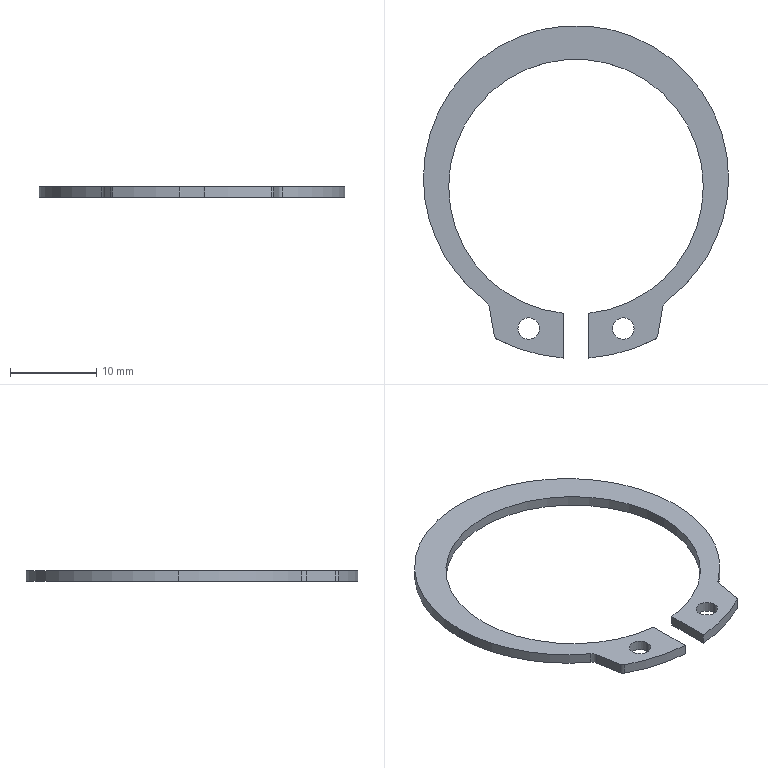Part | SolidWorks | features BaseBody 1 | 1 solid | 22 faces | box 35.48 x 38.644 x 1.2 mm | volume 408.802 mm3 | cylinder 16 | plane 6 | commonest cylinder face diameters 2.5 x4 29.6 x3 35.48 x3 1 x2 2 x2 39.96 x2
STEP:
#1=CARTESIAN_POINT('',(-4.25,-17.488,0.));
#2=VERTEX_POINT('',#1);
#3=CARTESIAN_POINT('',(-6.75,-17.488,0.));
#4=VERTEX_POINT('',#3);
#5=CARTESIAN_POINT('',(-5.5,-17.488,0.));
#6=DIRECTION('',(0.,0.,-1.));
#7=DIRECTION('',(1.,0.,0.));
#8=AXIS2_PLACEMENT_3D('',#5,#6,#7);
#9=CIRCLE('',#8,1.25);
#10=EDGE_CURVE('',#2,#4,#9,.T.);
#11=ORIENTED_EDGE('',*,*,#10,.T.);
#12=CARTESIAN_POINT('',(-6.75,-17.488,1.2));
#13=VERTEX_POINT('',#12);
#14=CARTESIAN_POINT('',(-6.75,-17.488,0.));
#15=DIRECTION('',(0.,0.,1.));
#16=VECTOR('',#15,1000.);
#17=LINE('',#14,#16);
#18=EDGE_CURVE('',#4,#13,#17,.T.);
#19=ORIENTED_EDGE('',*,*,#18,.T.);
#20=CARTESIAN_POINT('',(-4.25,-17.488,1.2));
#21=VERTEX_POINT('',#20);
#22=CARTESIAN_POINT('',(-5.5,-17.488,1.2));
#23=DIRECTION('',(0.,0.,-1.));
#24=DIRECTION('',(1.,0.,0.));
#25=AXIS2_PLACEMENT_3D('',#22,#23,#24);
#26=CIRCLE('',#25,1.25);
#27=EDGE_CURVE('',#21,#13,#26,.T.);
#28=ORIENTED_EDGE('',*,*,#27,.F.);
#29=CARTESIAN_POINT('',(-4.25,-17.488,0.));
#30=DIRECTION('',(0.,0.,1.));
#31=VECTOR('',#30,1000.);
#32=LINE('',#29,#31);
#33=EDGE_CURVE('',#2,#21,#32,.T.);
#34=ORIENTED_EDGE('',*,*,#33,.F.);
#35=EDGE_LOOP('',(#11,#19,#28,#34));
#36=FACE_OUTER_BOUND('',#35,.T.);
#37=CARTESIAN_POINT('',(-5.5,-17.488,0.));
#38=DIRECTION('',(0.,0.,1.));
#39=DIRECTION('',(1.,0.,0.));
#40=AXIS2_PLACEMENT_3D('',#37,#38,#39);
#41=CYLINDRICAL_SURFACE('',#40,1.25);
#42=ADVANCED_FACE('',(#36),#41,.F.);
#43=CARTESIAN_POINT('',(6.75,-17.488,0.));
#44=VERTEX_POINT('',#43);
#45=CARTESIAN_POINT('',(4.25,-17.488,0.));
#46=VERTEX_POINT('',#45);
#47=CARTESIAN_POINT('',(5.5,-17.488,0.));
#48=DIRECTION('',(0.,0.,-1.));
#49=DIRECTION('',(1.,0.,0.));
#50=AXIS2_PLACEMENT_3D('',#47,#48,#49);
#51=CIRCLE('',#50,1.25);
#52=EDGE_CURVE('',#44,#46,#51,.T.);
#53=ORIENTED_EDGE('',*,*,#52,.T.);
#54=CARTESIAN_POINT('',(4.25,-17.488,1.2));
#55=VERTEX_POINT('',#54);
#56=CARTESIAN_POINT('',(4.25,-17.488,0.));
#57=DIRECTION('',(0.,0.,1.));
#58=VECTOR('',#57,1000.);
#59=LINE('',#56,#58);
#60=EDGE_CURVE('',#46,#55,#59,.T.);
#61=ORIENTED_EDGE('',*,*,#60,.T.);
#62=CARTESIAN_POINT('',(6.75,-17.488,1.2));
#63=VERTEX_POINT('',#62);
#64=CARTESIAN_POINT('',(5.5,-17.488,1.2));
#65=DIRECTION('',(0.,0.,-1.));
#66=DIRECTION('',(1.,0.,0.));
#67=AXIS2_PLACEMENT_3D('',#64,#65,#66);
#68=CIRCLE('',#67,1.25);
#69=EDGE_CURVE('',#63,#55,#68,.T.);
#70=ORIENTED_EDGE('',*,*,#69,.F.);
#71=CARTESIAN_POINT('',(6.75,-17.488,0.));
#72=DIRECTION('',(0.,0.,1.));
#73=VECTOR('',#72,1000.);
#74=LINE('',#71,#73);
#75=EDGE_CURVE('',#44,#63,#74,.T.);
#76=ORIENTED_EDGE('',*,*,#75,.F.);
#77=EDGE_LOOP('',(#53,#61,#70,#76));
#78=FACE_OUTER_BOUND('',#77,.T.);
#79=CARTESIAN_POINT('',(5.5,-17.488,0.));
#80=DIRECTION('',(0.,0.,1.));
#81=DIRECTION('',(1.,0.,0.));
#82=AXIS2_PLACEMENT_3D('',#79,#80,#81);
#83=CYLINDRICAL_SURFACE('',#82,1.25);
#84=ADVANCED_FACE('',(#78),#83,.F.);
#85=CARTESIAN_POINT('',(17.74,0.,0.));
#86=VERTEX_POINT('',#85);
#87=CARTESIAN_POINT('',(-17.74,0.,0.));
#88=VERTEX_POINT('',#87);
#89=CARTESIAN_POINT('',(0.,0.,0.));
#90=DIRECTION('',(0.,0.,1.));
#91=DIRECTION('',(1.,0.,0.));
#92=AXIS2_PLACEMENT_3D('',#89,#90,#91);
#93=CIRCLE('',#92,17.74);
#94=EDGE_CURVE('',#86,#88,#93,.T.);
#95=ORIENTED_EDGE('',*,*,#94,.T.);
#96=CARTESIAN_POINT('',(-17.74,0.,1.2));
#97=VERTEX_POINT('',#96);
#98=CARTESIAN_POINT('',(-17.74,0.,0.));
#99=DIRECTION('',(0.,0.,1.));
#100=VECTOR('',#99,1000.);
#101=LINE('',#98,#100);
#102=EDGE_CURVE('',#88,#97,#101,.T.);
#103=ORIENTED_EDGE('',*,*,#102,.T.);
#104=CARTESIAN_POINT('',(17.74,0.,1.2));
#105=VERTEX_POINT('',#104);
#106=CARTESIAN_POINT('',(0.,0.,1.2));
#107=DIRECTION('',(0.,0.,-1.));
#108=DIRECTION('',(1.,0.,0.));
#109=AXIS2_PLACEMENT_3D('',#106,#107,#108);
#110=CIRCLE('',#109,17.74);
#111=EDGE_CURVE('',#97,#105,#110,.T.);
#112=ORIENTED_EDGE('',*,*,#111,.T.);
#113=CARTESIAN_POINT('',(17.74,0.,0.));
#114=DIRECTION('',(0.,0.,1.));
#115=VECTOR('',#114,1000.);
#116=LINE('',#113,#115);
#117=EDGE_CURVE('',#86,#105,#116,.T.);
#118=ORIENTED_EDGE('',*,*,#117,.F.);
#119=EDGE_LOOP('',(#95,#103,#112,#118));
#120=FACE_OUTER_BOUND('',#119,.T.);
#121=CARTESIAN_POINT('',(0.,0.,0.));
#122=DIRECTION('',(0.,0.,1.));
#123=DIRECTION('',(1.,0.,0.));
#124=AXIS2_PLACEMENT_3D('',#121,#122,#123);
#125=CYLINDRICAL_SURFACE('',#124,17.74);
#126=ADVANCED_FACE('',(#120),#125,.T.);
#127=CARTESIAN_POINT('',(10.493,-14.304,0.));
#128=VERTEX_POINT('',#127);
#129=CARTESIAN_POINT('',(0.,0.,0.));
#130=DIRECTION('',(0.,0.,1.));
#131=DIRECTION('',(1.,0.,0.));
#132=AXIS2_PLACEMENT_3D('',#129,#130,#131);
#133=CIRCLE('',#132,17.74);
#134=EDGE_CURVE('',#128,#86,#133,.T.);
#135=ORIENTED_EDGE('',*,*,#134,.T.);
#136=ORIENTED_EDGE('',*,*,#117,.T.);
#137=CARTESIAN_POINT('',(10.493,-14.304,1.2));
#138=VERTEX_POINT('',#137);
#139=CARTESIAN_POINT('',(0.,0.,1.2));
#140=DIRECTION('',(0.,0.,-1.));
#141=DIRECTION('',(1.,0.,0.));
#142=AXIS2_PLACEMENT_3D('',#139,#140,#141);
#143=CIRCLE('',#142,17.74);
#144=EDGE_CURVE('',#105,#138,#143,.T.);
#145=ORIENTED_EDGE('',*,*,#144,.T.);
#146=CARTESIAN_POINT('',(10.493,-14.304,0.));
#147=DIRECTION('',(0.,0.,-1.));
#148=VECTOR('',#147,1000.);
#149=LINE('',#146,#148);
#150=EDGE_CURVE('',#138,#128,#149,.T.);
#151=ORIENTED_EDGE('',*,*,#150,.T.);
#152=EDGE_LOOP('',(#135,#136,#145,#151));
#153=FACE_OUTER_BOUND('',#152,.T.);
#154=CARTESIAN_POINT('',(0.,0.,0.));
#155=DIRECTION('',(0.,0.,1.));
#156=DIRECTION('',(1.,0.,0.));
#157=AXIS2_PLACEMENT_3D('',#154,#155,#156);
#158=CYLINDRICAL_SURFACE('',#157,17.74);
#159=ADVANCED_FACE('',(#153),#158,.T.);
#160=CARTESIAN_POINT('',(-1.5,-15.704,0.));
#161=VERTEX_POINT('',#160);
#162=CARTESIAN_POINT('',(-14.8,-0.98,0.));
#163=VERTEX_POINT('',#162);
#164=CARTESIAN_POINT('',(0.,-0.98,0.));
#165=DIRECTION('',(0.,0.,-1.));
#166=DIRECTION('',(1.,0.,0.));
#167=AXIS2_PLACEMENT_3D('',#164,#165,#166);
#168=CIRCLE('',#167,14.8);
#169=EDGE_CURVE('',#161,#163,#168,.T.);
#170=ORIENTED_EDGE('',*,*,#169,.T.);
#171=CARTESIAN_POINT('',(-14.8,-0.98,1.2));
#172=VERTEX_POINT('',#171);
#173=CARTESIAN_POINT('',(-14.8,-0.98,0.));
#174=DIRECTION('',(0.,0.,1.));
#175=VECTOR('',#174,1000.);
#176=LINE('',#173,#175);
#177=EDGE_CURVE('',#163,#172,#176,.T.);
#178=ORIENTED_EDGE('',*,*,#177,.T.);
#179=CARTESIAN_POINT('',(-1.5,-15.704,1.2));
#180=VERTEX_POINT('',#179);
#181=CARTESIAN_POINT('',(0.,-0.98,1.2));
#182=DIRECTION('',(0.,0.,-1.));
#183=DIRECTION('',(1.,0.,0.));
#184=AXIS2_PLACEMENT_3D('',#181,#182,#183);
#185=CIRCLE('',#184,14.8);
#186=EDGE_CURVE('',#180,#172,#185,.T.);
#187=ORIENTED_EDGE('',*,*,#186,.F.);
#188=CARTESIAN_POINT('',(-1.5,-15.704,0.));
#189=DIRECTION('',(0.,0.,1.));
#190=VECTOR('',#189,1000.);
#191=LINE('',#188,#190);
#192=EDGE_CURVE('',#161,#180,#191,.T.);
#193=ORIENTED_EDGE('',*,*,#192,.F.);
#194=EDGE_LOOP('',(#170,#178,#187,#193));
#195=FACE_OUTER_BOUND('',#194,.T.);
#196=CARTESIAN_POINT('',(0.,-0.98,0.));
#197=DIRECTION('',(0.,0.,1.));
#198=DIRECTION('',(1.,0.,0.));
#199=AXIS2_PLACEMENT_3D('',#196,#197,#198);
#200=CYLINDRICAL_SURFACE('',#199,14.8);
#201=ADVANCED_FACE('',(#195),#200,.F.);
#202=ORIENTED_EDGE('',*,*,#177,.F.);
#203=CARTESIAN_POINT('',(14.8,-0.98,0.));
#204=VERTEX_POINT('',#203);
#205=CARTESIAN_POINT('',(0.,-0.98,0.));
#206=DIRECTION('',(0.,0.,-1.));
#207=DIRECTION('',(1.,0.,0.));
#208=AXIS2_PLACEMENT_3D('',#205,#206,#207);
#209=CIRCLE('',#208,14.8);
#210=EDGE_CURVE('',#163,#204,#209,.T.);
#211=ORIENTED_EDGE('',*,*,#210,.T.);
#212=CARTESIAN_POINT('',(14.8,-0.98,1.2));
#213=VERTEX_POINT('',#212);
#214=CARTESIAN_POINT('',(14.8,-0.98,0.));
#215=DIRECTION('',(0.,0.,1.));
#216=VECTOR('',#215,1000.);
#217=LINE('',#214,#216);
#218=EDGE_CURVE('',#204,#213,#217,.T.);
#219=ORIENTED_EDGE('',*,*,#218,.T.);
#220=CARTESIAN_POINT('',(0.,-0.98,1.2));
#221=DIRECTION('',(0.,0.,-1.));
#222=DIRECTION('',(1.,0.,0.));
#223=AXIS2_PLACEMENT_3D('',#220,#221,#222);
#224=CIRCLE('',#223,14.8);
#225=EDGE_CURVE('',#172,#213,#224,.T.);
#226=ORIENTED_EDGE('',*,*,#225,.F.);
#227=EDGE_LOOP('',(#202,#211,#219,#226));
#228=FACE_OUTER_BOUND('',#227,.T.);
#229=CARTESIAN_POINT('',(0.,-0.98,0.));
#230=DIRECTION('',(0.,0.,1.));
#231=DIRECTION('',(1.,0.,0.));
#232=AXIS2_PLACEMENT_3D('',#229,#230,#231);
#233=CYLINDRICAL_SURFACE('',#232,14.8);
#234=ADVANCED_FACE('',(#228),#233,.F.);
#235=ORIENTED_EDGE('',*,*,#10,.F.);
#236=CARTESIAN_POINT('',(-5.5,-17.488,0.));
#237=DIRECTION('',(0.,0.,-1.));
#238=DIRECTION('',(1.,0.,0.));
#239=AXIS2_PLACEMENT_3D('',#236,#237,#238);
#240=CIRCLE('',#239,1.25);
#241=EDGE_CURVE('',#4,#2,#240,.T.);
#242=ORIENTED_EDGE('',*,*,#241,.F.);
#243=EDGE_LOOP('',(#235,#242));
#244=FACE_BOUND('',#243,.T.);
#245=ORIENTED_EDGE('',*,*,#52,.F.);
#246=CARTESIAN_POINT('',(5.5,-17.488,0.));
#247=DIRECTION('',(0.,0.,-1.));
#248=DIRECTION('',(1.,0.,0.));
#249=AXIS2_PLACEMENT_3D('',#246,#247,#248);
#250=CIRCLE('',#249,1.25);
#251=EDGE_CURVE('',#46,#44,#250,.T.);
#252=ORIENTED_EDGE('',*,*,#251,.F.);
#253=EDGE_LOOP('',(#245,#252));
#254=FACE_BOUND('',#253,.T.);
#255=CARTESIAN_POINT('',(-9.5,-18.339,0.));
#256=VERTEX_POINT('',#255);
#257=CARTESIAN_POINT('',(-9.239,-18.696,0.));
#258=VERTEX_POINT('',#257);
#259=CARTESIAN_POINT('',(-9.008,-18.253,0.));
#260=DIRECTION('',(0.,0.,1.));
#261=DIRECTION('',(1.,0.,0.));
#262=AXIS2_PLACEMENT_3D('',#259,#260,#261);
#263=CIRCLE('',#262,0.5);
#264=EDGE_CURVE('',#256,#258,#263,.T.);
#265=ORIENTED_EDGE('',*,*,#264,.F.);
#266=CARTESIAN_POINT('',(-10.1,-14.936,0.));
#267=VERTEX_POINT('',#266);
#268=CARTESIAN_POINT('',(-10.1,-14.936,0.));
#269=DIRECTION('',(0.1736,-0.9848,0.));
#270=VECTOR('',#269,1000.);
#271=LINE('',#268,#270);
#272=EDGE_CURVE('',#267,#256,#271,.T.);
#273=ORIENTED_EDGE('',*,*,#272,.F.);
#274=CARTESIAN_POINT('',(-10.493,-14.304,0.));
#275=VERTEX_POINT('',#274);
#276=CARTESIAN_POINT('',(-11.085,-15.11,0.));
#277=DIRECTION('',(0.,0.,-1.));
#278=DIRECTION('',(1.,0.,0.));
#279=AXIS2_PLACEMENT_3D('',#276,#277,#278);
#280=CIRCLE('',#279,1.);
#281=EDGE_CURVE('',#275,#267,#280,.T.);
#282=ORIENTED_EDGE('',*,*,#281,.F.);
#283=CARTESIAN_POINT('',(0.,0.,0.));
#284=DIRECTION('',(0.,0.,1.));
#285=DIRECTION('',(1.,0.,0.));
#286=AXIS2_PLACEMENT_3D('',#283,#284,#285);
#287=CIRCLE('',#286,17.74);
#288=EDGE_CURVE('',#88,#275,#287,.T.);
#289=ORIENTED_EDGE('',*,*,#288,.F.);
#290=ORIENTED_EDGE('',*,*,#94,.F.);
#291=ORIENTED_EDGE('',*,*,#134,.F.);
#292=CARTESIAN_POINT('',(10.1,-14.936,0.));
#293=VERTEX_POINT('',#292);
#294=CARTESIAN_POINT('',(11.085,-15.11,0.));
#295=DIRECTION('',(0.,0.,-1.));
#296=DIRECTION('',(1.,0.,0.));
#297=AXIS2_PLACEMENT_3D('',#294,#295,#296);
#298=CIRCLE('',#297,1.);
#299=EDGE_CURVE('',#293,#128,#298,.T.);
#300=ORIENTED_EDGE('',*,*,#299,.F.);
#301=CARTESIAN_POINT('',(9.5,-18.339,0.));
#302=VERTEX_POINT('',#301);
#303=CARTESIAN_POINT('',(9.5,-18.339,0.));
#304=DIRECTION('',(0.1736,0.9848,0.));
#305=VECTOR('',#304,1000.);
#306=LINE('',#303,#305);
#307=EDGE_CURVE('',#302,#293,#306,.T.);
#308=ORIENTED_EDGE('',*,*,#307,.F.);
#309=CARTESIAN_POINT('',(9.239,-18.696,0.));
#310=VERTEX_POINT('',#309);
#311=CARTESIAN_POINT('',(9.008,-18.253,0.));
#312=DIRECTION('',(0.,0.,1.));
#313=DIRECTION('',(1.,0.,0.));
#314=AXIS2_PLACEMENT_3D('',#311,#312,#313);
#315=CIRCLE('',#314,0.5);
#316=EDGE_CURVE('',#310,#302,#315,.T.);
#317=ORIENTED_EDGE('',*,*,#316,.F.);
#318=CARTESIAN_POINT('',(1.5,-20.904,0.));
#319=VERTEX_POINT('',#318);
#320=CARTESIAN_POINT('',(0.,-0.98,0.));
#321=DIRECTION('',(0.,0.,1.));
#322=DIRECTION('',(1.,0.,0.));
#323=AXIS2_PLACEMENT_3D('',#320,#321,#322);
#324=CIRCLE('',#323,19.98);
#325=EDGE_CURVE('',#319,#310,#324,.T.);
#326=ORIENTED_EDGE('',*,*,#325,.F.);
#327=CARTESIAN_POINT('',(1.5,-15.704,0.));
#328=VERTEX_POINT('',#327);
#329=CARTESIAN_POINT('',(1.5,-2.899,0.));
#330=DIRECTION('',(0.,-1.,0.));
#331=VECTOR('',#330,1000.);
#332=LINE('',#329,#331);
#333=EDGE_CURVE('',#328,#319,#332,.T.);
#334=ORIENTED_EDGE('',*,*,#333,.F.);
#335=CARTESIAN_POINT('',(0.,-0.98,0.));
#336=DIRECTION('',(0.,0.,-1.));
#337=DIRECTION('',(1.,0.,0.));
#338=AXIS2_PLACEMENT_3D('',#335,#336,#337);
#339=CIRCLE('',#338,14.8);
#340=EDGE_CURVE('',#204,#328,#339,.T.);
#341=ORIENTED_EDGE('',*,*,#340,.F.);
#342=ORIENTED_EDGE('',*,*,#210,.F.);
#343=ORIENTED_EDGE('',*,*,#169,.F.);
#344=CARTESIAN_POINT('',(-1.5,-20.904,0.));
#345=VERTEX_POINT('',#344);
#346=CARTESIAN_POINT('',(-1.5,-2.899,0.));
#347=DIRECTION('',(0.,1.,0.));
#348=VECTOR('',#347,1000.);
#349=LINE('',#346,#348);
#350=EDGE_CURVE('',#345,#161,#349,.T.);
#351=ORIENTED_EDGE('',*,*,#350,.F.);
#352=CARTESIAN_POINT('',(0.,-0.98,0.));
#353=DIRECTION('',(0.,0.,1.));
#354=DIRECTION('',(1.,0.,0.));
#355=AXIS2_PLACEMENT_3D('',#352,#353,#354);
#356=CIRCLE('',#355,19.98);
#357=EDGE_CURVE('',#258,#345,#356,.T.);
#358=ORIENTED_EDGE('',*,*,#357,.F.);
#359=EDGE_LOOP('',(#265,#273,#282,#289,#290,#291,#300,#308,#317,#326,#334,#341,#342,#343,#351,#358));
#360=FACE_OUTER_BOUND('',#359,.T.);
#361=CARTESIAN_POINT('',(0.,-2.899,0.));
#362=DIRECTION('',(0.,0.,1.));
#363=DIRECTION('',(1.,0.,0.));
#364=AXIS2_PLACEMENT_3D('',#361,#362,#363);
#365=PLANE('',#364);
#366=ADVANCED_FACE('',(#244,#254,#360),#365,.F.);
#367=ORIENTED_EDGE('',*,*,#18,.F.);
#368=ORIENTED_EDGE('',*,*,#241,.T.);
#369=ORIENTED_EDGE('',*,*,#33,.T.);
#370=CARTESIAN_POINT('',(-5.5,-17.488,1.2));
#371=DIRECTION('',(0.,0.,-1.));
#372=DIRECTION('',(1.,0.,0.));
#373=AXIS2_PLACEMENT_3D('',#370,#371,#372);
#374=CIRCLE('',#373,1.25);
#375=EDGE_CURVE('',#13,#21,#374,.T.);
#376=ORIENTED_EDGE('',*,*,#375,.F.);
#377=EDGE_LOOP('',(#367,#368,#369,#376));
#378=FACE_OUTER_BOUND('',#377,.T.);
#379=CARTESIAN_POINT('',(-5.5,-17.488,0.));
#380=DIRECTION('',(0.,0.,1.));
#381=DIRECTION('',(1.,0.,0.));
#382=AXIS2_PLACEMENT_3D('',#379,#380,#381);
#383=CYLINDRICAL_SURFACE('',#382,1.25);
#384=ADVANCED_FACE('',(#378),#383,.F.);
#385=ORIENTED_EDGE('',*,*,#60,.F.);
#386=ORIENTED_EDGE('',*,*,#251,.T.);
#387=ORIENTED_EDGE('',*,*,#75,.T.);
#388=CARTESIAN_POINT('',(5.5,-17.488,1.2));
#389=DIRECTION('',(0.,0.,-1.));
#390=DIRECTION('',(1.,0.,0.));
#391=AXIS2_PLACEMENT_3D('',#388,#389,#390);
#392=CIRCLE('',#391,1.25);
#393=EDGE_CURVE('',#55,#63,#392,.T.);
#394=ORIENTED_EDGE('',*,*,#393,.F.);
#395=EDGE_LOOP('',(#385,#386,#387,#394));
#396=FACE_OUTER_BOUND('',#395,.T.);
#397=CARTESIAN_POINT('',(5.5,-17.488,0.));
#398=DIRECTION('',(0.,0.,1.));
#399=DIRECTION('',(1.,0.,0.));
#400=AXIS2_PLACEMENT_3D('',#397,#398,#399);
#401=CYLINDRICAL_SURFACE('',#400,1.25);
#402=ADVANCED_FACE('',(#396),#401,.F.);
#403=ORIENTED_EDGE('',*,*,#357,.T.);
#404=CARTESIAN_POINT('',(-1.5,-20.904,1.2));
#405=VERTEX_POINT('',#404);
#406=CARTESIAN_POINT('',(-1.5,-20.904,0.));
#407=DIRECTION('',(0.,0.,1.));
#408=VECTOR('',#407,1000.);
#409=LINE('',#406,#408);
#410=EDGE_CURVE('',#345,#405,#409,.T.);
#411=ORIENTED_EDGE('',*,*,#410,.T.);
#412=CARTESIAN_POINT('',(-9.239,-18.696,1.2));
#413=VERTEX_POINT('',#412);
#414=CARTESIAN_POINT('',(0.,-0.98,1.2));
#415=DIRECTION('',(0.,0.,-1.));
#416=DIRECTION('',(1.,0.,0.));
#417=AXIS2_PLACEMENT_3D('',#414,#415,#416);
#418=CIRCLE('',#417,19.98);
#419=EDGE_CURVE('',#405,#413,#418,.T.);
#420=ORIENTED_EDGE('',*,*,#419,.T.);
#421=CARTESIAN_POINT('',(-9.239,-18.696,0.));
#422=DIRECTION('',(0.,0.,-1.));
#423=VECTOR('',#422,1000.);
#424=LINE('',#421,#423);
#425=EDGE_CURVE('',#413,#258,#424,.T.);
#426=ORIENTED_EDGE('',*,*,#425,.T.);
#427=EDGE_LOOP('',(#403,#411,#420,#426));
#428=FACE_OUTER_BOUND('',#427,.T.);
#429=CARTESIAN_POINT('',(0.,-0.98,0.));
#430=DIRECTION('',(0.,0.,1.));
#431=DIRECTION('',(1.,0.,0.));
#432=AXIS2_PLACEMENT_3D('',#429,#430,#431);
#433=CYLINDRICAL_SURFACE('',#432,19.98);
#434=ADVANCED_FACE('',(#428),#433,.T.);
#435=ORIENTED_EDGE('',*,*,#264,.T.);
#436=ORIENTED_EDGE('',*,*,#425,.F.);
#437=CARTESIAN_POINT('',(-9.5,-18.339,1.2));
#438=VERTEX_POINT('',#437);
#439=CARTESIAN_POINT('',(-9.008,-18.253,1.2));
#440=DIRECTION('',(0.,0.,-1.));
#441=DIRECTION('',(1.,0.,0.));
#442=AXIS2_PLACEMENT_3D('',#439,#440,#441);
#443=CIRCLE('',#442,0.5);
#444=EDGE_CURVE('',#413,#438,#443,.T.);
#445=ORIENTED_EDGE('',*,*,#444,.T.);
#446=CARTESIAN_POINT('',(-9.5,-18.339,0.));
#447=DIRECTION('',(0.,0.,-1.));
#448=VECTOR('',#447,1000.);
#449=LINE('',#446,#448);
#450=EDGE_CURVE('',#438,#256,#449,.T.);
#451=ORIENTED_EDGE('',*,*,#450,.T.);
#452=EDGE_LOOP('',(#435,#436,#445,#451));
#453=FACE_OUTER_BOUND('',#452,.T.);
#454=CARTESIAN_POINT('',(-9.008,-18.253,0.));
#455=DIRECTION('',(0.,0.,1.));
#456=DIRECTION('',(1.,0.,0.));
#457=AXIS2_PLACEMENT_3D('',#454,#455,#456);
#458=CYLINDRICAL_SURFACE('',#457,0.5);
#459=ADVANCED_FACE('',(#453),#458,.T.);
#460=ORIENTED_EDGE('',*,*,#272,.T.);
#461=ORIENTED_EDGE('',*,*,#450,.F.);
#462=CARTESIAN_POINT('',(-10.1,-14.936,1.2));
#463=VERTEX_POINT('',#462);
#464=CARTESIAN_POINT('',(-9.5,-18.339,1.2));
#465=DIRECTION('',(-0.1736,0.9848,0.));
#466=VECTOR('',#465,1000.);
#467=LINE('',#464,#466);
#468=EDGE_CURVE('',#438,#463,#467,.T.);
#469=ORIENTED_EDGE('',*,*,#468,.T.);
#470=CARTESIAN_POINT('',(-10.1,-14.936,0.));
#471=DIRECTION('',(0.,0.,-1.));
#472=VECTOR('',#471,1000.);
#473=LINE('',#470,#472);
#474=EDGE_CURVE('',#463,#267,#473,.T.);
#475=ORIENTED_EDGE('',*,*,#474,.T.);
#476=EDGE_LOOP('',(#460,#461,#469,#475));
#477=FACE_OUTER_BOUND('',#476,.T.);
#478=CARTESIAN_POINT('',(-9.5,-18.339,0.));
#479=DIRECTION('',(-0.9848,-0.1736,0.));
#480=DIRECTION('',(0.1736,-0.9848,0.));
#481=AXIS2_PLACEMENT_3D('',#478,#479,#480);
#482=PLANE('',#481);
#483=ADVANCED_FACE('',(#477),#482,.T.);
#484=CARTESIAN_POINT('',(-10.493,-14.304,1.2));
#485=VERTEX_POINT('',#484);
#486=CARTESIAN_POINT('',(-10.493,-14.304,0.));
#487=DIRECTION('',(0.,0.,1.));
#488=VECTOR('',#487,1000.);
#489=LINE('',#486,#488);
#490=EDGE_CURVE('',#275,#485,#489,.T.);
#491=ORIENTED_EDGE('',*,*,#490,.F.);
#492=ORIENTED_EDGE('',*,*,#281,.T.);
#493=ORIENTED_EDGE('',*,*,#474,.F.);
#494=CARTESIAN_POINT('',(-11.085,-15.11,1.2));
#495=DIRECTION('',(0.,0.,-1.));
#496=DIRECTION('',(1.,0.,0.));
#497=AXIS2_PLACEMENT_3D('',#494,#495,#496);
#498=CIRCLE('',#497,1.);
#499=EDGE_CURVE('',#485,#463,#498,.T.);
#500=ORIENTED_EDGE('',*,*,#499,.F.);
#501=EDGE_LOOP('',(#491,#492,#493,#500));
#502=FACE_OUTER_BOUND('',#501,.T.);
#503=CARTESIAN_POINT('',(-11.085,-15.11,0.));
#504=DIRECTION('',(0.,0.,1.));
#505=DIRECTION('',(1.,0.,0.));
#506=AXIS2_PLACEMENT_3D('',#503,#504,#505);
#507=CYLINDRICAL_SURFACE('',#506,1.);
#508=ADVANCED_FACE('',(#502),#507,.F.);
#509=ORIENTED_EDGE('',*,*,#102,.F.);
#510=ORIENTED_EDGE('',*,*,#288,.T.);
#511=ORIENTED_EDGE('',*,*,#490,.T.);
#512=CARTESIAN_POINT('',(0.,0.,1.2));
#513=DIRECTION('',(0.,0.,-1.));
#514=DIRECTION('',(1.,0.,0.));
#515=AXIS2_PLACEMENT_3D('',#512,#513,#514);
#516=CIRCLE('',#515,17.74);
#517=EDGE_CURVE('',#485,#97,#516,.T.);
#518=ORIENTED_EDGE('',*,*,#517,.T.);
#519=EDGE_LOOP('',(#509,#510,#511,#518));
#520=FACE_OUTER_BOUND('',#519,.T.);
#521=CARTESIAN_POINT('',(0.,0.,0.));
#522=DIRECTION('',(0.,0.,1.));
#523=DIRECTION('',(1.,0.,0.));
#524=AXIS2_PLACEMENT_3D('',#521,#522,#523);
#525=CYLINDRICAL_SURFACE('',#524,17.74);
#526=ADVANCED_FACE('',(#520),#525,.T.);
#527=CARTESIAN_POINT('',(10.1,-14.936,1.2));
#528=VERTEX_POINT('',#527);
#529=CARTESIAN_POINT('',(10.1,-14.936,0.));
#530=DIRECTION('',(0.,0.,1.));
#531=VECTOR('',#530,1000.);
#532=LINE('',#529,#531);
#533=EDGE_CURVE('',#293,#528,#532,.T.);
#534=ORIENTED_EDGE('',*,*,#533,.F.);
#535=ORIENTED_EDGE('',*,*,#299,.T.);
#536=ORIENTED_EDGE('',*,*,#150,.F.);
#537=CARTESIAN_POINT('',(11.085,-15.11,1.2));
#538=DIRECTION('',(0.,0.,-1.));
#539=DIRECTION('',(1.,0.,0.));
#540=AXIS2_PLACEMENT_3D('',#537,#538,#539);
#541=CIRCLE('',#540,1.);
#542=EDGE_CURVE('',#528,#138,#541,.T.);
#543=ORIENTED_EDGE('',*,*,#542,.F.);
#544=EDGE_LOOP('',(#534,#535,#536,#543));
#545=FACE_OUTER_BOUND('',#544,.T.);
#546=CARTESIAN_POINT('',(11.085,-15.11,0.));
#547=DIRECTION('',(0.,0.,1.));
#548=DIRECTION('',(1.,0.,0.));
#549=AXIS2_PLACEMENT_3D('',#546,#547,#548);
#550=CYLINDRICAL_SURFACE('',#549,1.);
#551=ADVANCED_FACE('',(#545),#550,.F.);
#552=ORIENTED_EDGE('',*,*,#307,.T.);
#553=ORIENTED_EDGE('',*,*,#533,.T.);
#554=CARTESIAN_POINT('',(9.5,-18.339,1.2));
#555=VERTEX_POINT('',#554);
#556=CARTESIAN_POINT('',(10.1,-14.936,1.2));
#557=DIRECTION('',(-0.1736,-0.9848,0.));
#558=VECTOR('',#557,1000.);
#559=LINE('',#556,#558);
#560=EDGE_CURVE('',#528,#555,#559,.T.);
#561=ORIENTED_EDGE('',*,*,#560,.T.);
#562=CARTESIAN_POINT('',(9.5,-18.339,0.));
#563=DIRECTION('',(0.,0.,-1.));
#564=VECTOR('',#563,1000.);
#565=LINE('',#562,#564);
#566=EDGE_CURVE('',#555,#302,#565,.T.);
#567=ORIENTED_EDGE('',*,*,#566,.T.);
#568=EDGE_LOOP('',(#552,#553,#561,#567));
#569=FACE_OUTER_BOUND('',#568,.T.);
#570=CARTESIAN_POINT('',(10.1,-14.936,0.));
#571=DIRECTION('',(0.9848,-0.1736,0.));
#572=DIRECTION('',(0.1736,0.9848,0.));
#573=AXIS2_PLACEMENT_3D('',#570,#571,#572);
#574=PLANE('',#573);
#575=ADVANCED_FACE('',(#569),#574,.T.);
#576=ORIENTED_EDGE('',*,*,#316,.T.);
#577=ORIENTED_EDGE('',*,*,#566,.F.);
#578=CARTESIAN_POINT('',(9.239,-18.696,1.2));
#579=VERTEX_POINT('',#578);
#580=CARTESIAN_POINT('',(9.008,-18.253,1.2));
#581=DIRECTION('',(0.,0.,-1.));
#582=DIRECTION('',(1.,0.,0.));
#583=AXIS2_PLACEMENT_3D('',#580,#581,#582);
#584=CIRCLE('',#583,0.5);
#585=EDGE_CURVE('',#555,#579,#584,.T.);
#586=ORIENTED_EDGE('',*,*,#585,.T.);
#587=CARTESIAN_POINT('',(9.239,-18.696,0.));
#588=DIRECTION('',(0.,0.,-1.));
#589=VECTOR('',#588,1000.);
#590=LINE('',#587,#589);
#591=EDGE_CURVE('',#579,#310,#590,.T.);
#592=ORIENTED_EDGE('',*,*,#591,.T.);
#593=EDGE_LOOP('',(#576,#577,#586,#592));
#594=FACE_OUTER_BOUND('',#593,.T.);
#595=CARTESIAN_POINT('',(9.008,-18.253,0.));
#596=DIRECTION('',(0.,0.,1.));
#597=DIRECTION('',(1.,0.,0.));
#598=AXIS2_PLACEMENT_3D('',#595,#596,#597);
#599=CYLINDRICAL_SURFACE('',#598,0.5);
#600=ADVANCED_FACE('',(#594),#599,.T.);
#601=ORIENTED_EDGE('',*,*,#325,.T.);
#602=ORIENTED_EDGE('',*,*,#591,.F.);
#603=CARTESIAN_POINT('',(1.5,-20.904,1.2));
#604=VERTEX_POINT('',#603);
#605=CARTESIAN_POINT('',(0.,-0.98,1.2));
#606=DIRECTION('',(0.,0.,-1.));
#607=DIRECTION('',(1.,0.,0.));
#608=AXIS2_PLACEMENT_3D('',#605,#606,#607);
#609=CIRCLE('',#608,19.98);
#610=EDGE_CURVE('',#579,#604,#609,.T.);
#611=ORIENTED_EDGE('',*,*,#610,.T.);
#612=CARTESIAN_POINT('',(1.5,-20.904,0.));
#613=DIRECTION('',(0.,0.,-1.));
#614=VECTOR('',#613,1000.);
#615=LINE('',#612,#614);
#616=EDGE_CURVE('',#604,#319,#615,.T.);
#617=ORIENTED_EDGE('',*,*,#616,.T.);
#618=EDGE_LOOP('',(#601,#602,#611,#617));
#619=FACE_OUTER_BOUND('',#618,.T.);
#620=CARTESIAN_POINT('',(0.,-0.98,0.));
#621=DIRECTION('',(0.,0.,1.));
#622=DIRECTION('',(1.,0.,0.));
#623=AXIS2_PLACEMENT_3D('',#620,#621,#622);
#624=CYLINDRICAL_SURFACE('',#623,19.98);
#625=ADVANCED_FACE('',(#619),#624,.T.);
#626=ORIENTED_EDGE('',*,*,#333,.T.);
#627=ORIENTED_EDGE('',*,*,#616,.F.);
#628=CARTESIAN_POINT('',(1.5,-15.704,1.2));
#629=VERTEX_POINT('',#628);
#630=CARTESIAN_POINT('',(1.5,-20.904,1.2));
#631=DIRECTION('',(0.,1.,0.));
#632=VECTOR('',#631,1000.);
#633=LINE('',#630,#632);
#634=EDGE_CURVE('',#604,#629,#633,.T.);
#635=ORIENTED_EDGE('',*,*,#634,.T.);
#636=CARTESIAN_POINT('',(1.5,-15.704,0.));
#637=DIRECTION('',(0.,0.,-1.));
#638=VECTOR('',#637,1000.);
#639=LINE('',#636,#638);
#640=EDGE_CURVE('',#629,#328,#639,.T.);
#641=ORIENTED_EDGE('',*,*,#640,.T.);
#642=EDGE_LOOP('',(#626,#627,#635,#641));
#643=FACE_OUTER_BOUND('',#642,.T.);
#644=CARTESIAN_POINT('',(1.5,-20.904,0.));
#645=DIRECTION('',(-1.,0.,0.));
#646=DIRECTION('',(0.,-1.,0.));
#647=AXIS2_PLACEMENT_3D('',#644,#645,#646);
#648=PLANE('',#647);
#649=ADVANCED_FACE('',(#643),#648,.T.);
#650=ORIENTED_EDGE('',*,*,#218,.F.);
#651=ORIENTED_EDGE('',*,*,#340,.T.);
#652=ORIENTED_EDGE('',*,*,#640,.F.);
#653=CARTESIAN_POINT('',(0.,-0.98,1.2));
#654=DIRECTION('',(0.,0.,-1.));
#655=DIRECTION('',(1.,0.,0.));
#656=AXIS2_PLACEMENT_3D('',#653,#654,#655);
#657=CIRCLE('',#656,14.8);
#658=EDGE_CURVE('',#213,#629,#657,.T.);
#659=ORIENTED_EDGE('',*,*,#658,.F.);
#660=EDGE_LOOP('',(#650,#651,#652,#659));
#661=FACE_OUTER_BOUND('',#660,.T.);
#662=CARTESIAN_POINT('',(0.,-0.98,0.));
#663=DIRECTION('',(0.,0.,1.));
#664=DIRECTION('',(1.,0.,0.));
#665=AXIS2_PLACEMENT_3D('',#662,#663,#664);
#666=CYLINDRICAL_SURFACE('',#665,14.8);
#667=ADVANCED_FACE('',(#661),#666,.F.);
#668=ORIENTED_EDGE('',*,*,#350,.T.);
#669=ORIENTED_EDGE('',*,*,#192,.T.);
#670=CARTESIAN_POINT('',(-1.5,-15.704,1.2));
#671=DIRECTION('',(0.,-1.,0.));
#672=VECTOR('',#671,1000.);
#673=LINE('',#670,#672);
#674=EDGE_CURVE('',#180,#405,#673,.T.);
#675=ORIENTED_EDGE('',*,*,#674,.T.);
#676=ORIENTED_EDGE('',*,*,#410,.F.);
#677=EDGE_LOOP('',(#668,#669,#675,#676));
#678=FACE_OUTER_BOUND('',#677,.T.);
#679=CARTESIAN_POINT('',(-1.5,-15.704,0.));
#680=DIRECTION('',(1.,0.,0.));
#681=DIRECTION('',(0.,1.,0.));
#682=AXIS2_PLACEMENT_3D('',#679,#680,#681);
#683=PLANE('',#682);
#684=ADVANCED_FACE('',(#678),#683,.T.);
#685=ORIENTED_EDGE('',*,*,#27,.T.);
#686=ORIENTED_EDGE('',*,*,#375,.T.);
#687=EDGE_LOOP('',(#685,#686));
#688=FACE_BOUND('',#687,.T.);
#689=ORIENTED_EDGE('',*,*,#69,.T.);
#690=ORIENTED_EDGE('',*,*,#393,.T.);
#691=EDGE_LOOP('',(#689,#690));
#692=FACE_BOUND('',#691,.T.);
#693=ORIENTED_EDGE('',*,*,#499,.T.);
#694=ORIENTED_EDGE('',*,*,#468,.F.);
#695=ORIENTED_EDGE('',*,*,#444,.F.);
#696=ORIENTED_EDGE('',*,*,#419,.F.);
#697=ORIENTED_EDGE('',*,*,#674,.F.);
#698=ORIENTED_EDGE('',*,*,#186,.T.);
#699=ORIENTED_EDGE('',*,*,#225,.T.);
#700=ORIENTED_EDGE('',*,*,#658,.T.);
#701=ORIENTED_EDGE('',*,*,#634,.F.);
#702=ORIENTED_EDGE('',*,*,#610,.F.);
#703=ORIENTED_EDGE('',*,*,#585,.F.);
#704=ORIENTED_EDGE('',*,*,#560,.F.);
#705=ORIENTED_EDGE('',*,*,#542,.T.);
#706=ORIENTED_EDGE('',*,*,#144,.F.);
#707=ORIENTED_EDGE('',*,*,#111,.F.);
#708=ORIENTED_EDGE('',*,*,#517,.F.);
#709=EDGE_LOOP('',(#693,#694,#695,#696,#697,#698,#699,#700,#701,#702,#703,#704,#705,#706,#707,#708));
#710=FACE_OUTER_BOUND('',#709,.T.);
#711=CARTESIAN_POINT('',(0.,-2.899,1.2));
#712=DIRECTION('',(0.,0.,1.));
#713=DIRECTION('',(1.,0.,0.));
#714=AXIS2_PLACEMENT_3D('',#711,#712,#713);
#715=PLANE('',#714);
#716=ADVANCED_FACE('',(#688,#692,#710),#715,.T.);
#717=CLOSED_SHELL('',(#42,#84,#126,#159,#201,#234,#366,#384,#402,#434,#459,#483,#508,#526,#551,#575,#600,#625,#649,#667,#684,#716));
#718=MANIFOLD_SOLID_BREP('',#717);
#719=CARTESIAN_POINT('',(0.,0.,0.));
#720=DIRECTION('',(0.,0.,1.));
#721=DIRECTION('',(1.,0.,0.));
#722=AXIS2_PLACEMENT_3D('',#719,#720,#721);
#723=(LENGTH_UNIT()NAMED_UNIT(*)SI_UNIT(.MILLI.,.METRE.));
#724=UNCERTAINTY_MEASURE_WITH_UNIT(LENGTH_MEASURE(0.00001),#723,'','');
#725=(NAMED_UNIT(*)PLANE_ANGLE_UNIT()SI_UNIT($,.RADIAN.));
#726=(NAMED_UNIT(*)SI_UNIT($,.STERADIAN.)SOLID_ANGLE_UNIT());
#727=(GEOMETRIC_REPRESENTATION_CONTEXT(3)GLOBAL_UNCERTAINTY_ASSIGNED_CONTEXT((#724))GLOBAL_UNIT_ASSIGNED_CONTEXT((#723,#725,#726))REPRESENTATION_CONTEXT('',''));
#728=ADVANCED_BREP_SHAPE_REPRESENTATION('',(#718,#722),#727);